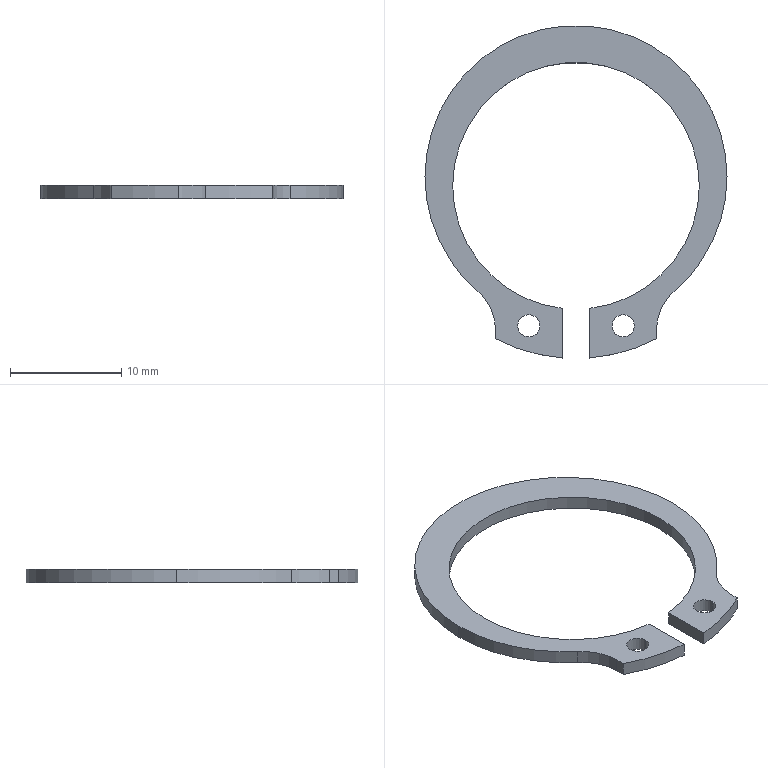Part | NX | features BREP 1 | 1 solid | 20 faces | box 27.2 x 29.93 x 1.2 mm | volume 263.5 mm3 | cylinder 14 | plane 6 | commonest cylinder face diameters 2 x4 22.2 x3 27.2 x3 9 x2 31.1 x2
STEP:
#1=CARTESIAN_POINT('',(3.25,-13.433,-1.2));
#2=VERTEX_POINT('',#1);
#3=CARTESIAN_POINT('',(5.25,-13.433,-1.2));
#4=VERTEX_POINT('',#3);
#5=CARTESIAN_POINT('',(4.25,-13.433,-1.2));
#6=DIRECTION('',(0.,0.,1.));
#7=DIRECTION('',(-1.,0.,0.));
#8=AXIS2_PLACEMENT_3D('',#5,#6,#7);
#9=CIRCLE('',#8,1.);
#10=EDGE_CURVE('',#2,#4,#9,.T.);
#11=ORIENTED_EDGE('',*,*,#10,.F.);
#12=CARTESIAN_POINT('',(3.25,-13.433,0.));
#13=VERTEX_POINT('',#12);
#14=CARTESIAN_POINT('',(3.25,-13.433,-1.2));
#15=DIRECTION('',(0.,0.,1.));
#16=VECTOR('',#15,1000.);
#17=LINE('',#14,#16);
#18=EDGE_CURVE('',#2,#13,#17,.T.);
#19=ORIENTED_EDGE('',*,*,#18,.T.);
#20=CARTESIAN_POINT('',(5.25,-13.433,0.));
#21=VERTEX_POINT('',#20);
#22=CARTESIAN_POINT('',(4.25,-13.433,0.));
#23=DIRECTION('',(0.,0.,1.));
#24=DIRECTION('',(-1.,0.,0.));
#25=AXIS2_PLACEMENT_3D('',#22,#23,#24);
#26=CIRCLE('',#25,1.);
#27=EDGE_CURVE('',#13,#21,#26,.T.);
#28=ORIENTED_EDGE('',*,*,#27,.T.);
#29=CARTESIAN_POINT('',(5.25,-13.433,-1.2));
#30=DIRECTION('',(0.,0.,1.));
#31=VECTOR('',#30,1000.);
#32=LINE('',#29,#31);
#33=EDGE_CURVE('',#4,#21,#32,.T.);
#34=ORIENTED_EDGE('',*,*,#33,.F.);
#35=EDGE_LOOP('',(#11,#19,#28,#34));
#36=FACE_BOUND('',#35,.T.);
#37=CARTESIAN_POINT('',(4.25,-13.433,-1.2));
#38=DIRECTION('',(0.,0.,1.));
#39=DIRECTION('',(-1.,0.,0.));
#40=AXIS2_PLACEMENT_3D('',#37,#38,#39);
#41=CYLINDRICAL_SURFACE('',#40,1.);
#42=ADVANCED_FACE('',(#36),#41,.F.);
#43=CARTESIAN_POINT('',(-5.25,-13.433,-1.2));
#44=VERTEX_POINT('',#43);
#45=CARTESIAN_POINT('',(-3.25,-13.433,-1.2));
#46=VERTEX_POINT('',#45);
#47=CARTESIAN_POINT('',(-4.25,-13.433,-1.2));
#48=DIRECTION('',(0.,0.,1.));
#49=DIRECTION('',(1.,0.,0.));
#50=AXIS2_PLACEMENT_3D('',#47,#48,#49);
#51=CIRCLE('',#50,1.);
#52=EDGE_CURVE('',#44,#46,#51,.T.);
#53=ORIENTED_EDGE('',*,*,#52,.F.);
#54=CARTESIAN_POINT('',(-5.25,-13.433,0.));
#55=VERTEX_POINT('',#54);
#56=CARTESIAN_POINT('',(-5.25,-13.433,-1.2));
#57=DIRECTION('',(0.,0.,1.));
#58=VECTOR('',#57,1000.);
#59=LINE('',#56,#58);
#60=EDGE_CURVE('',#44,#55,#59,.T.);
#61=ORIENTED_EDGE('',*,*,#60,.T.);
#62=CARTESIAN_POINT('',(-3.25,-13.433,0.));
#63=VERTEX_POINT('',#62);
#64=CARTESIAN_POINT('',(-4.25,-13.433,0.));
#65=DIRECTION('',(0.,0.,1.));
#66=DIRECTION('',(1.,0.,0.));
#67=AXIS2_PLACEMENT_3D('',#64,#65,#66);
#68=CIRCLE('',#67,1.);
#69=EDGE_CURVE('',#55,#63,#68,.T.);
#70=ORIENTED_EDGE('',*,*,#69,.T.);
#71=CARTESIAN_POINT('',(-3.25,-13.433,-1.2));
#72=DIRECTION('',(0.,0.,1.));
#73=VECTOR('',#72,1000.);
#74=LINE('',#71,#73);
#75=EDGE_CURVE('',#46,#63,#74,.T.);
#76=ORIENTED_EDGE('',*,*,#75,.F.);
#77=EDGE_LOOP('',(#53,#61,#70,#76));
#78=FACE_BOUND('',#77,.T.);
#79=CARTESIAN_POINT('',(-4.25,-13.433,-1.2));
#80=DIRECTION('',(0.,0.,1.));
#81=DIRECTION('',(-1.,0.,0.));
#82=AXIS2_PLACEMENT_3D('',#79,#80,#81);
#83=CYLINDRICAL_SURFACE('',#82,1.);
#84=ADVANCED_FACE('',(#78),#83,.F.);
#85=CARTESIAN_POINT('',(-1.25,-11.859,-1.2));
#86=VERTEX_POINT('',#85);
#87=CARTESIAN_POINT('',(-11.1,-0.83,-1.2));
#88=VERTEX_POINT('',#87);
#89=CARTESIAN_POINT('',(0.,-0.83,-1.2));
#90=DIRECTION('',(0.,0.,-1.));
#91=DIRECTION('',(1.,0.,0.));
#92=AXIS2_PLACEMENT_3D('',#89,#90,#91);
#93=CIRCLE('',#92,11.1);
#94=EDGE_CURVE('',#86,#88,#93,.T.);
#95=ORIENTED_EDGE('',*,*,#94,.T.);
#96=CARTESIAN_POINT('',(-11.1,-0.83,0.));
#97=VERTEX_POINT('',#96);
#98=CARTESIAN_POINT('',(-11.1,-0.83,-1.2));
#99=DIRECTION('',(0.,0.,1.));
#100=VECTOR('',#99,1000.);
#101=LINE('',#98,#100);
#102=EDGE_CURVE('',#88,#97,#101,.T.);
#103=ORIENTED_EDGE('',*,*,#102,.T.);
#104=CARTESIAN_POINT('',(-1.25,-11.859,0.));
#105=VERTEX_POINT('',#104);
#106=CARTESIAN_POINT('',(0.,-0.83,0.));
#107=DIRECTION('',(0.,0.,-1.));
#108=DIRECTION('',(1.,0.,0.));
#109=AXIS2_PLACEMENT_3D('',#106,#107,#108);
#110=CIRCLE('',#109,11.1);
#111=EDGE_CURVE('',#105,#97,#110,.T.);
#112=ORIENTED_EDGE('',*,*,#111,.F.);
#113=CARTESIAN_POINT('',(-1.25,-11.859,-1.2));
#114=DIRECTION('',(0.,0.,1.));
#115=VECTOR('',#114,1000.);
#116=LINE('',#113,#115);
#117=EDGE_CURVE('',#86,#105,#116,.T.);
#118=ORIENTED_EDGE('',*,*,#117,.F.);
#119=EDGE_LOOP('',(#95,#103,#112,#118));
#120=FACE_BOUND('',#119,.T.);
#121=CARTESIAN_POINT('',(0.,-0.83,-1.2));
#122=DIRECTION('',(0.,0.,1.));
#123=DIRECTION('',(-1.,0.,0.));
#124=AXIS2_PLACEMENT_3D('',#121,#122,#123);
#125=CYLINDRICAL_SURFACE('',#124,11.1);
#126=ADVANCED_FACE('',(#120),#125,.F.);
#127=ORIENTED_EDGE('',*,*,#102,.F.);
#128=CARTESIAN_POINT('',(11.1,-0.83,-1.2));
#129=VERTEX_POINT('',#128);
#130=CARTESIAN_POINT('',(0.,-0.83,-1.2));
#131=DIRECTION('',(0.,0.,-1.));
#132=DIRECTION('',(1.,0.,0.));
#133=AXIS2_PLACEMENT_3D('',#130,#131,#132);
#134=CIRCLE('',#133,11.1);
#135=EDGE_CURVE('',#88,#129,#134,.T.);
#136=ORIENTED_EDGE('',*,*,#135,.T.);
#137=CARTESIAN_POINT('',(11.1,-0.83,0.));
#138=VERTEX_POINT('',#137);
#139=CARTESIAN_POINT('',(11.1,-0.83,-1.2));
#140=DIRECTION('',(0.,0.,1.));
#141=VECTOR('',#140,1000.);
#142=LINE('',#139,#141);
#143=EDGE_CURVE('',#129,#138,#142,.T.);
#144=ORIENTED_EDGE('',*,*,#143,.T.);
#145=CARTESIAN_POINT('',(0.,-0.83,0.));
#146=DIRECTION('',(0.,0.,-1.));
#147=DIRECTION('',(1.,0.,0.));
#148=AXIS2_PLACEMENT_3D('',#145,#146,#147);
#149=CIRCLE('',#148,11.1);
#150=EDGE_CURVE('',#97,#138,#149,.T.);
#151=ORIENTED_EDGE('',*,*,#150,.F.);
#152=EDGE_LOOP('',(#127,#136,#144,#151));
#153=FACE_BOUND('',#152,.T.);
#154=CARTESIAN_POINT('',(0.,-0.83,-1.2));
#155=DIRECTION('',(0.,0.,1.));
#156=DIRECTION('',(-1.,0.,0.));
#157=AXIS2_PLACEMENT_3D('',#154,#155,#156);
#158=CYLINDRICAL_SURFACE('',#157,11.1);
#159=ADVANCED_FACE('',(#153),#158,.F.);
#160=CARTESIAN_POINT('',(13.6,0.,-1.2));
#161=VERTEX_POINT('',#160);
#162=CARTESIAN_POINT('',(-13.6,0.,-1.2));
#163=VERTEX_POINT('',#162);
#164=CARTESIAN_POINT('',(0.,0.,-1.2));
#165=DIRECTION('',(0.,0.,1.));
#166=DIRECTION('',(1.,0.,0.));
#167=AXIS2_PLACEMENT_3D('',#164,#165,#166);
#168=CIRCLE('',#167,13.6);
#169=EDGE_CURVE('',#161,#163,#168,.T.);
#170=ORIENTED_EDGE('',*,*,#169,.T.);
#171=CARTESIAN_POINT('',(-13.6,0.,0.));
#172=VERTEX_POINT('',#171);
#173=CARTESIAN_POINT('',(-13.6,0.,-1.2));
#174=DIRECTION('',(0.,0.,1.));
#175=VECTOR('',#174,1000.);
#176=LINE('',#173,#175);
#177=EDGE_CURVE('',#163,#172,#176,.T.);
#178=ORIENTED_EDGE('',*,*,#177,.T.);
#179=CARTESIAN_POINT('',(13.6,0.,0.));
#180=VERTEX_POINT('',#179);
#181=CARTESIAN_POINT('',(0.,0.,0.));
#182=DIRECTION('',(0.,0.,1.));
#183=DIRECTION('',(1.,0.,0.));
#184=AXIS2_PLACEMENT_3D('',#181,#182,#183);
#185=CIRCLE('',#184,13.6);
#186=EDGE_CURVE('',#180,#172,#185,.T.);
#187=ORIENTED_EDGE('',*,*,#186,.F.);
#188=CARTESIAN_POINT('',(13.6,0.,-1.2));
#189=DIRECTION('',(0.,0.,1.));
#190=VECTOR('',#189,1000.);
#191=LINE('',#188,#190);
#192=EDGE_CURVE('',#161,#180,#191,.T.);
#193=ORIENTED_EDGE('',*,*,#192,.F.);
#194=EDGE_LOOP('',(#170,#178,#187,#193));
#195=FACE_BOUND('',#194,.T.);
#196=CARTESIAN_POINT('',(0.,0.,-1.2));
#197=DIRECTION('',(0.,0.,1.));
#198=DIRECTION('',(-1.,0.,0.));
#199=AXIS2_PLACEMENT_3D('',#196,#197,#198);
#200=CYLINDRICAL_SURFACE('',#199,13.6);
#201=ADVANCED_FACE('',(#195),#200,.T.);
#202=CARTESIAN_POINT('',(8.829,-10.345,-1.2));
#203=VERTEX_POINT('',#202);
#204=CARTESIAN_POINT('',(0.,0.,-1.2));
#205=DIRECTION('',(0.,0.,1.));
#206=DIRECTION('',(1.,0.,0.));
#207=AXIS2_PLACEMENT_3D('',#204,#205,#206);
#208=CIRCLE('',#207,13.6);
#209=EDGE_CURVE('',#203,#161,#208,.T.);
#210=ORIENTED_EDGE('',*,*,#209,.T.);
#211=ORIENTED_EDGE('',*,*,#192,.T.);
#212=CARTESIAN_POINT('',(8.829,-10.345,0.));
#213=VERTEX_POINT('',#212);
#214=CARTESIAN_POINT('',(0.,0.,0.));
#215=DIRECTION('',(0.,0.,1.));
#216=DIRECTION('',(1.,0.,0.));
#217=AXIS2_PLACEMENT_3D('',#214,#215,#216);
#218=CIRCLE('',#217,13.6);
#219=EDGE_CURVE('',#213,#180,#218,.T.);
#220=ORIENTED_EDGE('',*,*,#219,.F.);
#221=CARTESIAN_POINT('',(8.829,-10.345,-1.2));
#222=DIRECTION('',(0.,0.,-1.));
#223=VECTOR('',#222,1000.);
#224=LINE('',#221,#223);
#225=EDGE_CURVE('',#213,#203,#224,.T.);
#226=ORIENTED_EDGE('',*,*,#225,.T.);
#227=EDGE_LOOP('',(#210,#211,#220,#226));
#228=FACE_BOUND('',#227,.T.);
#229=CARTESIAN_POINT('',(0.,0.,-1.2));
#230=DIRECTION('',(0.,0.,1.));
#231=DIRECTION('',(-1.,0.,0.));
#232=AXIS2_PLACEMENT_3D('',#229,#230,#231);
#233=CYLINDRICAL_SURFACE('',#232,13.6);
#234=ADVANCED_FACE('',(#228),#233,.T.);
#235=ORIENTED_EDGE('',*,*,#177,.F.);
#236=CARTESIAN_POINT('',(-8.829,-10.345,-1.2));
#237=VERTEX_POINT('',#236);
#238=CARTESIAN_POINT('',(0.,0.,-1.2));
#239=DIRECTION('',(0.,0.,1.));
#240=DIRECTION('',(1.,0.,0.));
#241=AXIS2_PLACEMENT_3D('',#238,#239,#240);
#242=CIRCLE('',#241,13.6);
#243=EDGE_CURVE('',#163,#237,#242,.T.);
#244=ORIENTED_EDGE('',*,*,#243,.T.);
#245=CARTESIAN_POINT('',(-8.829,-10.345,0.));
#246=VERTEX_POINT('',#245);
#247=CARTESIAN_POINT('',(-8.829,-10.345,-1.2));
#248=DIRECTION('',(0.,0.,1.));
#249=VECTOR('',#248,1000.);
#250=LINE('',#247,#249);
#251=EDGE_CURVE('',#237,#246,#250,.T.);
#252=ORIENTED_EDGE('',*,*,#251,.T.);
#253=CARTESIAN_POINT('',(0.,0.,0.));
#254=DIRECTION('',(0.,0.,1.));
#255=DIRECTION('',(1.,0.,0.));
#256=AXIS2_PLACEMENT_3D('',#253,#254,#255);
#257=CIRCLE('',#256,13.6);
#258=EDGE_CURVE('',#172,#246,#257,.T.);
#259=ORIENTED_EDGE('',*,*,#258,.F.);
#260=EDGE_LOOP('',(#235,#244,#252,#259));
#261=FACE_BOUND('',#260,.T.);
#262=CARTESIAN_POINT('',(0.,0.,-1.2));
#263=DIRECTION('',(0.,0.,1.));
#264=DIRECTION('',(-1.,0.,0.));
#265=AXIS2_PLACEMENT_3D('',#262,#263,#264);
#266=CYLINDRICAL_SURFACE('',#265,13.6);
#267=ADVANCED_FACE('',(#261),#266,.T.);
#268=CARTESIAN_POINT('',(7.25,-14.586,-1.2));
#269=VERTEX_POINT('',#268);
#270=CARTESIAN_POINT('',(7.25,-13.768,-1.2));
#271=VERTEX_POINT('',#270);
#272=CARTESIAN_POINT('',(7.25,-11.506,-1.2));
#273=DIRECTION('',(0.,1.,0.));
#274=VECTOR('',#273,1000.);
#275=LINE('',#272,#274);
#276=EDGE_CURVE('',#269,#271,#275,.T.);
#277=ORIENTED_EDGE('',*,*,#276,.T.);
#278=CARTESIAN_POINT('',(7.25,-13.768,0.));
#279=VERTEX_POINT('',#278);
#280=CARTESIAN_POINT('',(7.25,-13.768,0.));
#281=DIRECTION('',(0.,0.,1.));
#282=VECTOR('',#281,1000.);
#283=LINE('',#280,#282);
#284=EDGE_CURVE('',#271,#279,#283,.T.);
#285=ORIENTED_EDGE('',*,*,#284,.T.);
#286=CARTESIAN_POINT('',(7.25,-14.586,0.));
#287=VERTEX_POINT('',#286);
#288=CARTESIAN_POINT('',(7.25,-11.506,0.));
#289=DIRECTION('',(0.,1.,0.));
#290=VECTOR('',#289,1000.);
#291=LINE('',#288,#290);
#292=EDGE_CURVE('',#287,#279,#291,.T.);
#293=ORIENTED_EDGE('',*,*,#292,.F.);
#294=CARTESIAN_POINT('',(7.25,-14.586,-1.2));
#295=DIRECTION('',(0.,0.,1.));
#296=VECTOR('',#295,1000.);
#297=LINE('',#294,#296);
#298=EDGE_CURVE('',#269,#287,#297,.T.);
#299=ORIENTED_EDGE('',*,*,#298,.F.);
#300=EDGE_LOOP('',(#277,#285,#293,#299));
#301=FACE_BOUND('',#300,.T.);
#302=CARTESIAN_POINT('',(7.25,-11.506,-1.2));
#303=DIRECTION('',(1.,0.,0.));
#304=DIRECTION('',(0.,-1.,0.));
#305=AXIS2_PLACEMENT_3D('',#302,#303,#304);
#306=PLANE('',#305);
#307=ADVANCED_FACE('',(#301),#306,.T.);
#308=CARTESIAN_POINT('',(1.25,-16.33,0.));
#309=VERTEX_POINT('',#308);
#310=CARTESIAN_POINT('',(0.,-0.83,0.));
#311=DIRECTION('',(0.,0.,1.));
#312=DIRECTION('',(-1.,0.,0.));
#313=AXIS2_PLACEMENT_3D('',#310,#311,#312);
#314=CIRCLE('',#313,15.55);
#315=EDGE_CURVE('',#309,#287,#314,.T.);
#316=ORIENTED_EDGE('',*,*,#315,.F.);
#317=CARTESIAN_POINT('',(1.25,-16.33,-1.2));
#318=VERTEX_POINT('',#317);
#319=CARTESIAN_POINT('',(1.25,-16.33,-1.2));
#320=DIRECTION('',(0.,0.,1.));
#321=VECTOR('',#320,1000.);
#322=LINE('',#319,#321);
#323=EDGE_CURVE('',#318,#309,#322,.T.);
#324=ORIENTED_EDGE('',*,*,#323,.F.);
#325=CARTESIAN_POINT('',(0.,-0.83,-1.2));
#326=DIRECTION('',(0.,0.,1.));
#327=DIRECTION('',(-1.,0.,0.));
#328=AXIS2_PLACEMENT_3D('',#325,#326,#327);
#329=CIRCLE('',#328,15.55);
#330=EDGE_CURVE('',#318,#269,#329,.T.);
#331=ORIENTED_EDGE('',*,*,#330,.T.);
#332=ORIENTED_EDGE('',*,*,#298,.T.);
#333=EDGE_LOOP('',(#316,#324,#331,#332));
#334=FACE_BOUND('',#333,.T.);
#335=CARTESIAN_POINT('',(0.,-0.83,-1.2));
#336=DIRECTION('',(0.,0.,1.));
#337=DIRECTION('',(-1.,0.,0.));
#338=AXIS2_PLACEMENT_3D('',#335,#336,#337);
#339=CYLINDRICAL_SURFACE('',#338,15.55);
#340=ADVANCED_FACE('',(#334),#339,.T.);
#341=CARTESIAN_POINT('',(1.25,-11.859,0.));
#342=VERTEX_POINT('',#341);
#343=CARTESIAN_POINT('',(1.25,-16.33,0.));
#344=DIRECTION('',(0.,-1.,0.));
#345=VECTOR('',#344,1000.);
#346=LINE('',#343,#345);
#347=EDGE_CURVE('',#342,#309,#346,.T.);
#348=ORIENTED_EDGE('',*,*,#347,.F.);
#349=CARTESIAN_POINT('',(1.25,-11.859,-1.2));
#350=VERTEX_POINT('',#349);
#351=CARTESIAN_POINT('',(1.25,-11.859,-1.2));
#352=DIRECTION('',(0.,0.,1.));
#353=VECTOR('',#352,1000.);
#354=LINE('',#351,#353);
#355=EDGE_CURVE('',#350,#342,#354,.T.);
#356=ORIENTED_EDGE('',*,*,#355,.F.);
#357=CARTESIAN_POINT('',(1.25,-16.33,-1.2));
#358=DIRECTION('',(0.,-1.,0.));
#359=VECTOR('',#358,1000.);
#360=LINE('',#357,#359);
#361=EDGE_CURVE('',#350,#318,#360,.T.);
#362=ORIENTED_EDGE('',*,*,#361,.T.);
#363=ORIENTED_EDGE('',*,*,#323,.T.);
#364=EDGE_LOOP('',(#348,#356,#362,#363));
#365=FACE_BOUND('',#364,.T.);
#366=CARTESIAN_POINT('',(1.25,-16.33,-1.2));
#367=DIRECTION('',(-1.,0.,0.));
#368=DIRECTION('',(0.,-1.,0.));
#369=AXIS2_PLACEMENT_3D('',#366,#367,#368);
#370=PLANE('',#369);
#371=ADVANCED_FACE('',(#365),#370,.T.);
#372=ORIENTED_EDGE('',*,*,#143,.F.);
#373=CARTESIAN_POINT('',(0.,-0.83,-1.2));
#374=DIRECTION('',(0.,0.,-1.));
#375=DIRECTION('',(1.,0.,0.));
#376=AXIS2_PLACEMENT_3D('',#373,#374,#375);
#377=CIRCLE('',#376,11.1);
#378=EDGE_CURVE('',#129,#350,#377,.T.);
#379=ORIENTED_EDGE('',*,*,#378,.T.);
#380=ORIENTED_EDGE('',*,*,#355,.T.);
#381=CARTESIAN_POINT('',(0.,-0.83,0.));
#382=DIRECTION('',(0.,0.,-1.));
#383=DIRECTION('',(1.,0.,0.));
#384=AXIS2_PLACEMENT_3D('',#381,#382,#383);
#385=CIRCLE('',#384,11.1);
#386=EDGE_CURVE('',#138,#342,#385,.T.);
#387=ORIENTED_EDGE('',*,*,#386,.F.);
#388=EDGE_LOOP('',(#372,#379,#380,#387));
#389=FACE_BOUND('',#388,.T.);
#390=CARTESIAN_POINT('',(0.,-0.83,-1.2));
#391=DIRECTION('',(0.,0.,1.));
#392=DIRECTION('',(-1.,0.,0.));
#393=AXIS2_PLACEMENT_3D('',#390,#391,#392);
#394=CYLINDRICAL_SURFACE('',#393,11.1);
#395=ADVANCED_FACE('',(#389),#394,.F.);
#396=CARTESIAN_POINT('',(-1.25,-16.33,0.));
#397=VERTEX_POINT('',#396);
#398=CARTESIAN_POINT('',(-1.25,-16.33,0.));
#399=DIRECTION('',(0.,1.,0.));
#400=VECTOR('',#399,1000.);
#401=LINE('',#398,#400);
#402=EDGE_CURVE('',#397,#105,#401,.T.);
#403=ORIENTED_EDGE('',*,*,#402,.F.);
#404=CARTESIAN_POINT('',(-1.25,-16.33,-1.2));
#405=VERTEX_POINT('',#404);
#406=CARTESIAN_POINT('',(-1.25,-16.33,-1.2));
#407=DIRECTION('',(0.,0.,1.));
#408=VECTOR('',#407,1000.);
#409=LINE('',#406,#408);
#410=EDGE_CURVE('',#405,#397,#409,.T.);
#411=ORIENTED_EDGE('',*,*,#410,.F.);
#412=CARTESIAN_POINT('',(-1.25,-16.33,-1.2));
#413=DIRECTION('',(0.,1.,0.));
#414=VECTOR('',#413,1000.);
#415=LINE('',#412,#414);
#416=EDGE_CURVE('',#405,#86,#415,.T.);
#417=ORIENTED_EDGE('',*,*,#416,.T.);
#418=ORIENTED_EDGE('',*,*,#117,.T.);
#419=EDGE_LOOP('',(#403,#411,#417,#418));
#420=FACE_BOUND('',#419,.T.);
#421=CARTESIAN_POINT('',(-1.25,-16.33,-1.2));
#422=DIRECTION('',(1.,0.,0.));
#423=DIRECTION('',(0.,0.,-1.));
#424=AXIS2_PLACEMENT_3D('',#421,#422,#423);
#425=PLANE('',#424);
#426=ADVANCED_FACE('',(#420),#425,.T.);
#427=CARTESIAN_POINT('',(-7.25,-14.586,0.));
#428=VERTEX_POINT('',#427);
#429=CARTESIAN_POINT('',(0.,-0.83,0.));
#430=DIRECTION('',(0.,0.,1.));
#431=DIRECTION('',(1.,0.,0.));
#432=AXIS2_PLACEMENT_3D('',#429,#430,#431);
#433=CIRCLE('',#432,15.55);
#434=EDGE_CURVE('',#428,#397,#433,.T.);
#435=ORIENTED_EDGE('',*,*,#434,.F.);
#436=CARTESIAN_POINT('',(-7.25,-14.586,-1.2));
#437=VERTEX_POINT('',#436);
#438=CARTESIAN_POINT('',(-7.25,-14.586,-1.2));
#439=DIRECTION('',(0.,0.,1.));
#440=VECTOR('',#439,1000.);
#441=LINE('',#438,#440);
#442=EDGE_CURVE('',#437,#428,#441,.T.);
#443=ORIENTED_EDGE('',*,*,#442,.F.);
#444=CARTESIAN_POINT('',(0.,-0.83,-1.2));
#445=DIRECTION('',(0.,0.,1.));
#446=DIRECTION('',(1.,0.,0.));
#447=AXIS2_PLACEMENT_3D('',#444,#445,#446);
#448=CIRCLE('',#447,15.55);
#449=EDGE_CURVE('',#437,#405,#448,.T.);
#450=ORIENTED_EDGE('',*,*,#449,.T.);
#451=ORIENTED_EDGE('',*,*,#410,.T.);
#452=EDGE_LOOP('',(#435,#443,#450,#451));
#453=FACE_BOUND('',#452,.T.);
#454=CARTESIAN_POINT('',(0.,-0.83,-1.2));
#455=DIRECTION('',(0.,0.,1.));
#456=DIRECTION('',(-1.,0.,0.));
#457=AXIS2_PLACEMENT_3D('',#454,#455,#456);
#458=CYLINDRICAL_SURFACE('',#457,15.55);
#459=ADVANCED_FACE('',(#453),#458,.T.);
#460=CARTESIAN_POINT('',(-7.25,-13.768,0.));
#461=VERTEX_POINT('',#460);
#462=CARTESIAN_POINT('',(-7.25,-11.506,0.));
#463=DIRECTION('',(0.,-1.,0.));
#464=VECTOR('',#463,1000.);
#465=LINE('',#462,#464);
#466=EDGE_CURVE('',#461,#428,#465,.T.);
#467=ORIENTED_EDGE('',*,*,#466,.F.);
#468=CARTESIAN_POINT('',(-7.25,-13.768,-1.2));
#469=VERTEX_POINT('',#468);
#470=CARTESIAN_POINT('',(-7.25,-13.768,-1.2));
#471=DIRECTION('',(0.,0.,-1.));
#472=VECTOR('',#471,1000.);
#473=LINE('',#470,#472);
#474=EDGE_CURVE('',#461,#469,#473,.T.);
#475=ORIENTED_EDGE('',*,*,#474,.T.);
#476=CARTESIAN_POINT('',(-7.25,-11.506,-1.2));
#477=DIRECTION('',(0.,-1.,0.));
#478=VECTOR('',#477,1000.);
#479=LINE('',#476,#478);
#480=EDGE_CURVE('',#469,#437,#479,.T.);
#481=ORIENTED_EDGE('',*,*,#480,.T.);
#482=ORIENTED_EDGE('',*,*,#442,.T.);
#483=EDGE_LOOP('',(#467,#475,#481,#482));
#484=FACE_BOUND('',#483,.T.);
#485=CARTESIAN_POINT('',(-7.25,-11.506,-1.2));
#486=DIRECTION('',(-1.,0.,0.));
#487=DIRECTION('',(0.,0.,-1.));
#488=AXIS2_PLACEMENT_3D('',#485,#486,#487);
#489=PLANE('',#488);
#490=ADVANCED_FACE('',(#484),#489,.T.);
#491=ORIENTED_EDGE('',*,*,#209,.F.);
#492=CARTESIAN_POINT('',(11.75,-13.768,-1.2));
#493=DIRECTION('',(0.,0.,1.));
#494=DIRECTION('',(1.,0.,0.));
#495=AXIS2_PLACEMENT_3D('',#492,#493,#494);
#496=CIRCLE('',#495,4.5);
#497=EDGE_CURVE('',#203,#271,#496,.T.);
#498=ORIENTED_EDGE('',*,*,#497,.T.);
#499=ORIENTED_EDGE('',*,*,#276,.F.);
#500=ORIENTED_EDGE('',*,*,#330,.F.);
#501=ORIENTED_EDGE('',*,*,#361,.F.);
#502=ORIENTED_EDGE('',*,*,#378,.F.);
#503=ORIENTED_EDGE('',*,*,#135,.F.);
#504=ORIENTED_EDGE('',*,*,#94,.F.);
#505=ORIENTED_EDGE('',*,*,#416,.F.);
#506=ORIENTED_EDGE('',*,*,#449,.F.);
#507=ORIENTED_EDGE('',*,*,#480,.F.);
#508=CARTESIAN_POINT('',(-11.75,-13.768,-1.2));
#509=DIRECTION('',(0.,0.,1.));
#510=DIRECTION('',(1.,0.,0.));
#511=AXIS2_PLACEMENT_3D('',#508,#509,#510);
#512=CIRCLE('',#511,4.5);
#513=EDGE_CURVE('',#469,#237,#512,.T.);
#514=ORIENTED_EDGE('',*,*,#513,.T.);
#515=ORIENTED_EDGE('',*,*,#243,.F.);
#516=ORIENTED_EDGE('',*,*,#169,.F.);
#517=EDGE_LOOP('',(#491,#498,#499,#500,#501,#502,#503,#504,#505,#506,#507,#514,#515,#516));
#518=FACE_BOUND('',#517,.T.);
#519=CARTESIAN_POINT('',(4.25,-13.433,-1.2));
#520=DIRECTION('',(0.,0.,1.));
#521=DIRECTION('',(-1.,0.,0.));
#522=AXIS2_PLACEMENT_3D('',#519,#520,#521);
#523=CIRCLE('',#522,1.);
#524=EDGE_CURVE('',#4,#2,#523,.T.);
#525=ORIENTED_EDGE('',*,*,#524,.T.);
#526=ORIENTED_EDGE('',*,*,#10,.T.);
#527=EDGE_LOOP('',(#525,#526));
#528=FACE_BOUND('',#527,.T.);
#529=CARTESIAN_POINT('',(-4.25,-13.433,-1.2));
#530=DIRECTION('',(0.,0.,1.));
#531=DIRECTION('',(1.,0.,0.));
#532=AXIS2_PLACEMENT_3D('',#529,#530,#531);
#533=CIRCLE('',#532,1.);
#534=EDGE_CURVE('',#46,#44,#533,.T.);
#535=ORIENTED_EDGE('',*,*,#534,.T.);
#536=ORIENTED_EDGE('',*,*,#52,.T.);
#537=EDGE_LOOP('',(#535,#536));
#538=FACE_BOUND('',#537,.T.);
#539=CARTESIAN_POINT('',(0.,0.,-1.2));
#540=DIRECTION('',(0.,0.,1.));
#541=DIRECTION('',(0.,1.,0.));
#542=AXIS2_PLACEMENT_3D('',#539,#540,#541);
#543=PLANE('',#542);
#544=ADVANCED_FACE('',(#518,#528,#538),#543,.F.);
#545=ORIENTED_EDGE('',*,*,#292,.T.);
#546=CARTESIAN_POINT('',(11.75,-13.768,0.));
#547=DIRECTION('',(0.,0.,-1.));
#548=DIRECTION('',(1.,0.,0.));
#549=AXIS2_PLACEMENT_3D('',#546,#547,#548);
#550=CIRCLE('',#549,4.5);
#551=EDGE_CURVE('',#279,#213,#550,.T.);
#552=ORIENTED_EDGE('',*,*,#551,.T.);
#553=ORIENTED_EDGE('',*,*,#219,.T.);
#554=ORIENTED_EDGE('',*,*,#186,.T.);
#555=ORIENTED_EDGE('',*,*,#258,.T.);
#556=CARTESIAN_POINT('',(-11.75,-13.768,0.));
#557=DIRECTION('',(0.,0.,-1.));
#558=DIRECTION('',(1.,0.,0.));
#559=AXIS2_PLACEMENT_3D('',#556,#557,#558);
#560=CIRCLE('',#559,4.5);
#561=EDGE_CURVE('',#246,#461,#560,.T.);
#562=ORIENTED_EDGE('',*,*,#561,.T.);
#563=ORIENTED_EDGE('',*,*,#466,.T.);
#564=ORIENTED_EDGE('',*,*,#434,.T.);
#565=ORIENTED_EDGE('',*,*,#402,.T.);
#566=ORIENTED_EDGE('',*,*,#111,.T.);
#567=ORIENTED_EDGE('',*,*,#150,.T.);
#568=ORIENTED_EDGE('',*,*,#386,.T.);
#569=ORIENTED_EDGE('',*,*,#347,.T.);
#570=ORIENTED_EDGE('',*,*,#315,.T.);
#571=EDGE_LOOP('',(#545,#552,#553,#554,#555,#562,#563,#564,#565,#566,#567,#568,#569,#570));
#572=FACE_BOUND('',#571,.T.);
#573=CARTESIAN_POINT('',(4.25,-13.433,0.));
#574=DIRECTION('',(0.,0.,1.));
#575=DIRECTION('',(-1.,0.,0.));
#576=AXIS2_PLACEMENT_3D('',#573,#574,#575);
#577=CIRCLE('',#576,1.);
#578=EDGE_CURVE('',#21,#13,#577,.T.);
#579=ORIENTED_EDGE('',*,*,#578,.F.);
#580=ORIENTED_EDGE('',*,*,#27,.F.);
#581=EDGE_LOOP('',(#579,#580));
#582=FACE_BOUND('',#581,.T.);
#583=CARTESIAN_POINT('',(-4.25,-13.433,0.));
#584=DIRECTION('',(0.,0.,1.));
#585=DIRECTION('',(1.,0.,0.));
#586=AXIS2_PLACEMENT_3D('',#583,#584,#585);
#587=CIRCLE('',#586,1.);
#588=EDGE_CURVE('',#63,#55,#587,.T.);
#589=ORIENTED_EDGE('',*,*,#588,.F.);
#590=ORIENTED_EDGE('',*,*,#69,.F.);
#591=EDGE_LOOP('',(#589,#590));
#592=FACE_BOUND('',#591,.T.);
#593=CARTESIAN_POINT('',(0.,0.,0.));
#594=DIRECTION('',(0.,0.,1.));
#595=DIRECTION('',(0.,1.,0.));
#596=AXIS2_PLACEMENT_3D('',#593,#594,#595);
#597=PLANE('',#596);
#598=ADVANCED_FACE('',(#572,#582,#592),#597,.T.);
#599=ORIENTED_EDGE('',*,*,#60,.F.);
#600=ORIENTED_EDGE('',*,*,#534,.F.);
#601=ORIENTED_EDGE('',*,*,#75,.T.);
#602=ORIENTED_EDGE('',*,*,#588,.T.);
#603=EDGE_LOOP('',(#599,#600,#601,#602));
#604=FACE_BOUND('',#603,.T.);
#605=CARTESIAN_POINT('',(-4.25,-13.433,-1.2));
#606=DIRECTION('',(0.,0.,1.));
#607=DIRECTION('',(-1.,0.,0.));
#608=AXIS2_PLACEMENT_3D('',#605,#606,#607);
#609=CYLINDRICAL_SURFACE('',#608,1.);
#610=ADVANCED_FACE('',(#604),#609,.F.);
#611=ORIENTED_EDGE('',*,*,#18,.F.);
#612=ORIENTED_EDGE('',*,*,#524,.F.);
#613=ORIENTED_EDGE('',*,*,#33,.T.);
#614=ORIENTED_EDGE('',*,*,#578,.T.);
#615=EDGE_LOOP('',(#611,#612,#613,#614));
#616=FACE_BOUND('',#615,.T.);
#617=CARTESIAN_POINT('',(4.25,-13.433,-1.2));
#618=DIRECTION('',(0.,0.,1.));
#619=DIRECTION('',(-1.,0.,0.));
#620=AXIS2_PLACEMENT_3D('',#617,#618,#619);
#621=CYLINDRICAL_SURFACE('',#620,1.);
#622=ADVANCED_FACE('',(#616),#621,.F.);
#623=ORIENTED_EDGE('',*,*,#513,.F.);
#624=ORIENTED_EDGE('',*,*,#474,.F.);
#625=ORIENTED_EDGE('',*,*,#561,.F.);
#626=ORIENTED_EDGE('',*,*,#251,.F.);
#627=EDGE_LOOP('',(#623,#624,#625,#626));
#628=FACE_BOUND('',#627,.T.);
#629=CARTESIAN_POINT('',(-11.75,-13.768,-1.2));
#630=DIRECTION('',(0.,0.,1.));
#631=DIRECTION('',(-1.,0.,0.));
#632=AXIS2_PLACEMENT_3D('',#629,#630,#631);
#633=CYLINDRICAL_SURFACE('',#632,4.5);
#634=ADVANCED_FACE('',(#628),#633,.F.);
#635=ORIENTED_EDGE('',*,*,#497,.F.);
#636=ORIENTED_EDGE('',*,*,#225,.F.);
#637=ORIENTED_EDGE('',*,*,#551,.F.);
#638=ORIENTED_EDGE('',*,*,#284,.F.);
#639=EDGE_LOOP('',(#635,#636,#637,#638));
#640=FACE_BOUND('',#639,.T.);
#641=CARTESIAN_POINT('',(11.75,-13.768,-1.2));
#642=DIRECTION('',(0.,0.,1.));
#643=DIRECTION('',(-1.,0.,0.));
#644=AXIS2_PLACEMENT_3D('',#641,#642,#643);
#645=CYLINDRICAL_SURFACE('',#644,4.5);
#646=ADVANCED_FACE('',(#640),#645,.F.);
#647=CLOSED_SHELL('',(#42,#84,#126,#159,#201,#234,#267,#307,#340,#371,#395,#426,#459,#490,#544,#598,#610,#622,#634,#646));
#648=MANIFOLD_SOLID_BREP('',#647);
#649=(LENGTH_UNIT()NAMED_UNIT(*)SI_UNIT(.MILLI.,.METRE.));
#650=UNCERTAINTY_MEASURE_WITH_UNIT(LENGTH_MEASURE(0.00001),#649,'','');
#651=(NAMED_UNIT(*)PLANE_ANGLE_UNIT()SI_UNIT($,.RADIAN.));
#652=(NAMED_UNIT(*)SI_UNIT($,.STERADIAN.)SOLID_ANGLE_UNIT());
#653=(GEOMETRIC_REPRESENTATION_CONTEXT(3)GLOBAL_UNCERTAINTY_ASSIGNED_CONTEXT((#650))GLOBAL_UNIT_ASSIGNED_CONTEXT((#649,#651,#652))REPRESENTATION_CONTEXT('',''));
#654=ADVANCED_BREP_SHAPE_REPRESENTATION('',(#648),#653);